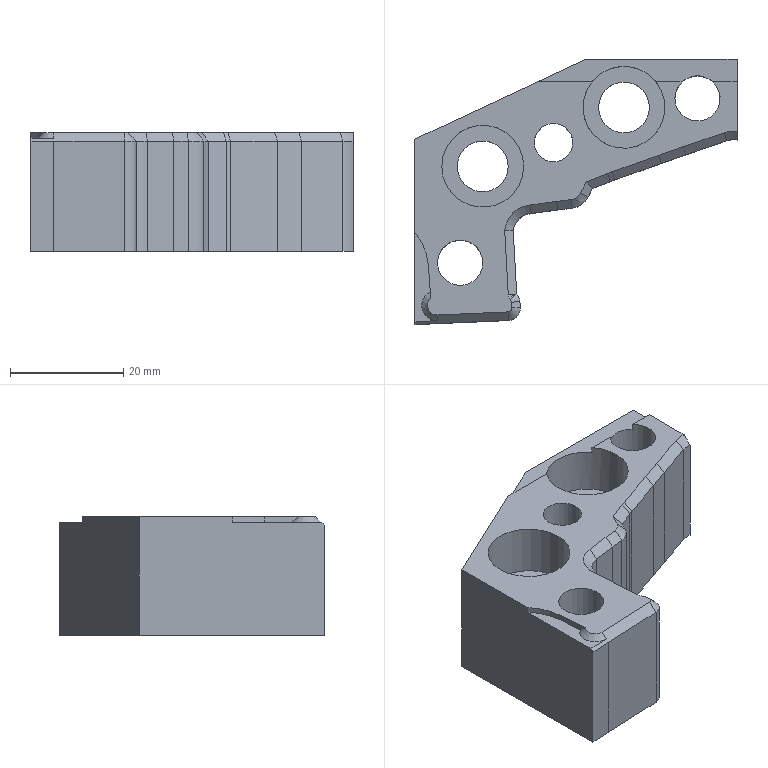Part | NX | features 23 2 | 1 solid | 57 faces | box 57 x 46.927 x 21 mm | volume 22755 mm3 | plane 37 | cylinder 13 | cone 7 | commonest cylinder face diameters 4.4 x2 8.001 x2 9 x2 14.5 x2 6.8 x1 6.899 x1